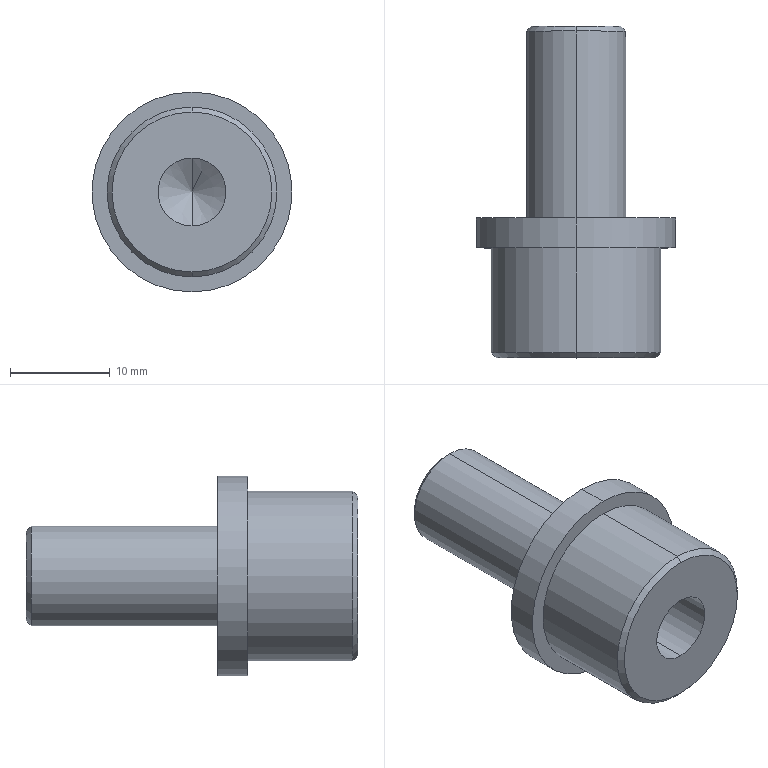Part | SolidWorks | features BaseBody 1 | 1 solid | 18 faces | box 20 x 33.2 x 20 mm | volume 4476 mm3 | cylinder 8 | cone 6 | plane 4 | commonest cylinder face diameters 6.8 x2 10 x2 17 x2 20 x2
STEP:
#1=CARTESIAN_POINT('',(0.,21.7,-5.));
#2=VERTEX_POINT('',#1);
#3=CARTESIAN_POINT('',(0.,21.7,5.));
#4=VERTEX_POINT('',#3);
#5=CARTESIAN_POINT('',(0.,21.7,0.));
#6=DIRECTION('',(0.,-1.,0.));
#7=DIRECTION('',(0.,0.,-1.));
#8=AXIS2_PLACEMENT_3D('',#5,#6,#7);
#9=CIRCLE('',#8,5.);
#10=EDGE_CURVE('',#2,#4,#9,.T.);
#11=ORIENTED_EDGE('',*,*,#10,.T.);
#12=CARTESIAN_POINT('',(0.,3.,5.));
#13=VERTEX_POINT('',#12);
#14=CARTESIAN_POINT('',(0.,22.2,5.));
#15=DIRECTION('',(0.,-1.,0.));
#16=VECTOR('',#15,1000.);
#17=LINE('',#14,#16);
#18=EDGE_CURVE('',#4,#13,#17,.T.);
#19=ORIENTED_EDGE('',*,*,#18,.T.);
#20=CARTESIAN_POINT('',(0.,3.,-5.));
#21=VERTEX_POINT('',#20);
#22=CARTESIAN_POINT('',(0.,3.,0.));
#23=DIRECTION('',(0.,1.,0.));
#24=DIRECTION('',(0.,0.,-1.));
#25=AXIS2_PLACEMENT_3D('',#22,#23,#24);
#26=CIRCLE('',#25,5.);
#27=EDGE_CURVE('',#13,#21,#26,.T.);
#28=ORIENTED_EDGE('',*,*,#27,.T.);
#29=CARTESIAN_POINT('',(0.,22.2,-5.));
#30=DIRECTION('',(0.,-1.,0.));
#31=VECTOR('',#30,1000.);
#32=LINE('',#29,#31);
#33=EDGE_CURVE('',#2,#21,#32,.T.);
#34=ORIENTED_EDGE('',*,*,#33,.F.);
#35=EDGE_LOOP('',(#11,#19,#28,#34));
#36=FACE_OUTER_BOUND('',#35,.T.);
#37=CARTESIAN_POINT('',(0.,22.2,0.));
#38=DIRECTION('',(0.,-1.,0.));
#39=DIRECTION('',(0.,0.,-1.));
#40=AXIS2_PLACEMENT_3D('',#37,#38,#39);
#41=CYLINDRICAL_SURFACE('',#40,5.);
#42=ADVANCED_FACE('',(#36),#41,.T.);
#43=CARTESIAN_POINT('',(0.,22.2,-4.5));
#44=VERTEX_POINT('',#43);
#45=CARTESIAN_POINT('',(0.,22.2,4.5));
#46=VERTEX_POINT('',#45);
#47=CARTESIAN_POINT('',(0.,22.2,0.));
#48=DIRECTION('',(0.,-1.,0.));
#49=DIRECTION('',(0.,0.,-1.));
#50=AXIS2_PLACEMENT_3D('',#47,#48,#49);
#51=CIRCLE('',#50,4.5);
#52=EDGE_CURVE('',#44,#46,#51,.T.);
#53=ORIENTED_EDGE('',*,*,#52,.T.);
#54=CARTESIAN_POINT('',(0.,21.7,5.));
#55=DIRECTION('',(0.,-0.7071,0.7071));
#56=VECTOR('',#55,1000.);
#57=LINE('',#54,#56);
#58=EDGE_CURVE('',#46,#4,#57,.T.);
#59=ORIENTED_EDGE('',*,*,#58,.T.);
#60=ORIENTED_EDGE('',*,*,#10,.F.);
#61=CARTESIAN_POINT('',(0.,21.7,-5.));
#62=DIRECTION('',(0.,-0.7071,-0.7071));
#63=VECTOR('',#62,1000.);
#64=LINE('',#61,#63);
#65=EDGE_CURVE('',#44,#2,#64,.T.);
#66=ORIENTED_EDGE('',*,*,#65,.F.);
#67=EDGE_LOOP('',(#53,#59,#60,#66));
#68=FACE_OUTER_BOUND('',#67,.T.);
#69=CARTESIAN_POINT('',(0.,21.7,0.));
#70=DIRECTION('',(0.,-1.,0.));
#71=DIRECTION('',(0.,0.,-1.));
#72=AXIS2_PLACEMENT_3D('',#69,#70,#71);
#73=CONICAL_SURFACE('',#72,5.,0.7854);
#74=ADVANCED_FACE('',(#68),#73,.T.);
#75=CARTESIAN_POINT('',(0.,3.,10.));
#76=VERTEX_POINT('',#75);
#77=CARTESIAN_POINT('',(0.,3.,-10.));
#78=VERTEX_POINT('',#77);
#79=CARTESIAN_POINT('',(0.,3.,0.));
#80=DIRECTION('',(0.,1.,0.));
#81=DIRECTION('',(0.,0.,-1.));
#82=AXIS2_PLACEMENT_3D('',#79,#80,#81);
#83=CIRCLE('',#82,10.);
#84=EDGE_CURVE('',#76,#78,#83,.T.);
#85=ORIENTED_EDGE('',*,*,#84,.F.);
#86=CARTESIAN_POINT('',(0.,0.,10.));
#87=VERTEX_POINT('',#86);
#88=CARTESIAN_POINT('',(0.,3.,10.));
#89=DIRECTION('',(0.,-1.,0.));
#90=VECTOR('',#89,1000.);
#91=LINE('',#88,#90);
#92=EDGE_CURVE('',#76,#87,#91,.T.);
#93=ORIENTED_EDGE('',*,*,#92,.T.);
#94=CARTESIAN_POINT('',(0.,0.,-10.));
#95=VERTEX_POINT('',#94);
#96=CARTESIAN_POINT('',(0.,0.,0.));
#97=DIRECTION('',(0.,1.,0.));
#98=DIRECTION('',(0.,0.,-1.));
#99=AXIS2_PLACEMENT_3D('',#96,#97,#98);
#100=CIRCLE('',#99,10.);
#101=EDGE_CURVE('',#87,#95,#100,.T.);
#102=ORIENTED_EDGE('',*,*,#101,.T.);
#103=CARTESIAN_POINT('',(0.,3.,-10.));
#104=DIRECTION('',(0.,-1.,0.));
#105=VECTOR('',#104,1000.);
#106=LINE('',#103,#105);
#107=EDGE_CURVE('',#78,#95,#106,.T.);
#108=ORIENTED_EDGE('',*,*,#107,.F.);
#109=EDGE_LOOP('',(#85,#93,#102,#108));
#110=FACE_OUTER_BOUND('',#109,.T.);
#111=CARTESIAN_POINT('',(0.,3.,0.));
#112=DIRECTION('',(0.,-1.,0.));
#113=DIRECTION('',(0.,0.,-1.));
#114=AXIS2_PLACEMENT_3D('',#111,#112,#113);
#115=CYLINDRICAL_SURFACE('',#114,10.);
#116=ADVANCED_FACE('',(#110),#115,.T.);
#117=CARTESIAN_POINT('',(0.,-10.5,8.5));
#118=VERTEX_POINT('',#117);
#119=CARTESIAN_POINT('',(0.,-10.5,-8.5));
#120=VERTEX_POINT('',#119);
#121=CARTESIAN_POINT('',(0.,-10.5,0.));
#122=DIRECTION('',(0.,1.,0.));
#123=DIRECTION('',(0.,0.,1.));
#124=AXIS2_PLACEMENT_3D('',#121,#122,#123);
#125=CIRCLE('',#124,8.5);
#126=EDGE_CURVE('',#118,#120,#125,.T.);
#127=ORIENTED_EDGE('',*,*,#126,.T.);
#128=CARTESIAN_POINT('',(0.,0.,-8.5));
#129=VERTEX_POINT('',#128);
#130=CARTESIAN_POINT('',(0.,-11.,-8.5));
#131=DIRECTION('',(0.,1.,0.));
#132=VECTOR('',#131,1000.);
#133=LINE('',#130,#132);
#134=EDGE_CURVE('',#120,#129,#133,.T.);
#135=ORIENTED_EDGE('',*,*,#134,.T.);
#136=CARTESIAN_POINT('',(0.,0.,8.5));
#137=VERTEX_POINT('',#136);
#138=CARTESIAN_POINT('',(0.,0.,0.));
#139=DIRECTION('',(0.,-1.,0.));
#140=DIRECTION('',(0.,0.,1.));
#141=AXIS2_PLACEMENT_3D('',#138,#139,#140);
#142=CIRCLE('',#141,8.5);
#143=EDGE_CURVE('',#129,#137,#142,.T.);
#144=ORIENTED_EDGE('',*,*,#143,.T.);
#145=CARTESIAN_POINT('',(0.,-11.,8.5));
#146=DIRECTION('',(0.,1.,0.));
#147=VECTOR('',#146,1000.);
#148=LINE('',#145,#147);
#149=EDGE_CURVE('',#118,#137,#148,.T.);
#150=ORIENTED_EDGE('',*,*,#149,.F.);
#151=EDGE_LOOP('',(#127,#135,#144,#150));
#152=FACE_OUTER_BOUND('',#151,.T.);
#153=CARTESIAN_POINT('',(0.,-11.,0.));
#154=DIRECTION('',(0.,1.,0.));
#155=DIRECTION('',(0.,0.,1.));
#156=AXIS2_PLACEMENT_3D('',#153,#154,#155);
#157=CYLINDRICAL_SURFACE('',#156,8.5);
#158=ADVANCED_FACE('',(#152),#157,.T.);
#159=CARTESIAN_POINT('',(0.,-11.,8.));
#160=VERTEX_POINT('',#159);
#161=CARTESIAN_POINT('',(0.,-11.,-8.));
#162=VERTEX_POINT('',#161);
#163=CARTESIAN_POINT('',(0.,-11.,0.));
#164=DIRECTION('',(0.,1.,0.));
#165=DIRECTION('',(0.,0.,1.));
#166=AXIS2_PLACEMENT_3D('',#163,#164,#165);
#167=CIRCLE('',#166,8.);
#168=EDGE_CURVE('',#160,#162,#167,.T.);
#169=ORIENTED_EDGE('',*,*,#168,.T.);
#170=CARTESIAN_POINT('',(0.,-10.5,-8.5));
#171=DIRECTION('',(0.,0.7071,-0.7071));
#172=VECTOR('',#171,1000.);
#173=LINE('',#170,#172);
#174=EDGE_CURVE('',#162,#120,#173,.T.);
#175=ORIENTED_EDGE('',*,*,#174,.T.);
#176=ORIENTED_EDGE('',*,*,#126,.F.);
#177=CARTESIAN_POINT('',(0.,-10.5,8.5));
#178=DIRECTION('',(0.,0.7071,0.7071));
#179=VECTOR('',#178,1000.);
#180=LINE('',#177,#179);
#181=EDGE_CURVE('',#160,#118,#180,.T.);
#182=ORIENTED_EDGE('',*,*,#181,.F.);
#183=EDGE_LOOP('',(#169,#175,#176,#182));
#184=FACE_OUTER_BOUND('',#183,.T.);
#185=CARTESIAN_POINT('',(0.,-10.5,0.));
#186=DIRECTION('',(0.,1.,0.));
#187=DIRECTION('',(0.,0.,1.));
#188=AXIS2_PLACEMENT_3D('',#185,#186,#187);
#189=CONICAL_SURFACE('',#188,8.5,0.7854);
#190=ADVANCED_FACE('',(#184),#189,.T.);
#191=CARTESIAN_POINT('',(0.,1.,3.4));
#192=VERTEX_POINT('',#191);
#193=CARTESIAN_POINT('',(0.,1.,-3.4));
#194=VERTEX_POINT('',#193);
#195=CARTESIAN_POINT('',(0.,1.,0.));
#196=DIRECTION('',(0.,-1.,0.));
#197=DIRECTION('',(0.,0.,-1.));
#198=AXIS2_PLACEMENT_3D('',#195,#196,#197);
#199=CIRCLE('',#198,3.4);
#200=EDGE_CURVE('',#192,#194,#199,.T.);
#201=ORIENTED_EDGE('',*,*,#200,.F.);
#202=CARTESIAN_POINT('',(0.,-11.,3.4));
#203=VERTEX_POINT('',#202);
#204=CARTESIAN_POINT('',(0.,-11.,3.4));
#205=DIRECTION('',(0.,-1.,0.));
#206=VECTOR('',#205,1000.);
#207=LINE('',#204,#206);
#208=EDGE_CURVE('',#192,#203,#207,.T.);
#209=ORIENTED_EDGE('',*,*,#208,.T.);
#210=CARTESIAN_POINT('',(0.,-11.,-3.4));
#211=VERTEX_POINT('',#210);
#212=CARTESIAN_POINT('',(0.,-11.,0.));
#213=DIRECTION('',(0.,1.,0.));
#214=DIRECTION('',(0.,0.,-1.));
#215=AXIS2_PLACEMENT_3D('',#212,#213,#214);
#216=CIRCLE('',#215,3.4);
#217=EDGE_CURVE('',#211,#203,#216,.T.);
#218=ORIENTED_EDGE('',*,*,#217,.F.);
#219=CARTESIAN_POINT('',(0.,-11.,-3.4));
#220=DIRECTION('',(0.,-1.,0.));
#221=VECTOR('',#220,1000.);
#222=LINE('',#219,#221);
#223=EDGE_CURVE('',#194,#211,#222,.T.);
#224=ORIENTED_EDGE('',*,*,#223,.F.);
#225=EDGE_LOOP('',(#201,#209,#218,#224));
#226=FACE_OUTER_BOUND('',#225,.T.);
#227=CARTESIAN_POINT('',(0.,-11.,0.));
#228=DIRECTION('',(0.,-1.,0.));
#229=DIRECTION('',(0.,0.,-1.));
#230=AXIS2_PLACEMENT_3D('',#227,#228,#229);
#231=CYLINDRICAL_SURFACE('',#230,3.4);
#232=ADVANCED_FACE('',(#226),#231,.F.);
#233=CARTESIAN_POINT('',(0.,3.043,0.));
#234=VERTEX_POINT('',#233);
#235=CARTESIAN_POINT('',(0.,1.,-3.4));
#236=DIRECTION('',(0.,-0.515,-0.8572));
#237=VECTOR('',#236,1000.);
#238=LINE('',#235,#237);
#239=EDGE_CURVE('',#234,#194,#238,.T.);
#240=ORIENTED_EDGE('',*,*,#239,.F.);
#241=CARTESIAN_POINT('',(0.,1.,3.4));
#242=DIRECTION('',(0.,-0.515,0.8572));
#243=VECTOR('',#242,1000.);
#244=LINE('',#241,#243);
#245=EDGE_CURVE('',#234,#192,#244,.T.);
#246=ORIENTED_EDGE('',*,*,#245,.T.);
#247=ORIENTED_EDGE('',*,*,#200,.T.);
#248=EDGE_LOOP('',(#240,#246,#247));
#249=FACE_OUTER_BOUND('',#248,.T.);
#250=CARTESIAN_POINT('',(0.,1.,0.));
#251=DIRECTION('',(0.,-1.,0.));
#252=DIRECTION('',(0.,0.,-1.));
#253=AXIS2_PLACEMENT_3D('',#250,#251,#252);
#254=CONICAL_SURFACE('',#253,3.4,1.03);
#255=ADVANCED_FACE('',(#249),#254,.F.);
#256=ORIENTED_EDGE('',*,*,#18,.F.);
#257=CARTESIAN_POINT('',(0.,21.7,0.));
#258=DIRECTION('',(0.,-1.,0.));
#259=DIRECTION('',(0.,0.,-1.));
#260=AXIS2_PLACEMENT_3D('',#257,#258,#259);
#261=CIRCLE('',#260,5.);
#262=EDGE_CURVE('',#4,#2,#261,.T.);
#263=ORIENTED_EDGE('',*,*,#262,.T.);
#264=ORIENTED_EDGE('',*,*,#33,.T.);
#265=CARTESIAN_POINT('',(0.,3.,0.));
#266=DIRECTION('',(0.,1.,0.));
#267=DIRECTION('',(0.,0.,-1.));
#268=AXIS2_PLACEMENT_3D('',#265,#266,#267);
#269=CIRCLE('',#268,5.);
#270=EDGE_CURVE('',#21,#13,#269,.T.);
#271=ORIENTED_EDGE('',*,*,#270,.T.);
#272=EDGE_LOOP('',(#256,#263,#264,#271));
#273=FACE_OUTER_BOUND('',#272,.T.);
#274=CARTESIAN_POINT('',(0.,22.2,0.));
#275=DIRECTION('',(0.,-1.,0.));
#276=DIRECTION('',(0.,0.,-1.));
#277=AXIS2_PLACEMENT_3D('',#274,#275,#276);
#278=CYLINDRICAL_SURFACE('',#277,5.);
#279=ADVANCED_FACE('',(#273),#278,.T.);
#280=CARTESIAN_POINT('',(0.,3.,0.));
#281=DIRECTION('',(0.,1.,0.));
#282=DIRECTION('',(0.,0.,-1.));
#283=AXIS2_PLACEMENT_3D('',#280,#281,#282);
#284=CIRCLE('',#283,10.);
#285=EDGE_CURVE('',#78,#76,#284,.T.);
#286=ORIENTED_EDGE('',*,*,#285,.T.);
#287=ORIENTED_EDGE('',*,*,#84,.T.);
#288=EDGE_LOOP('',(#286,#287));
#289=FACE_OUTER_BOUND('',#288,.T.);
#290=ORIENTED_EDGE('',*,*,#270,.F.);
#291=ORIENTED_EDGE('',*,*,#27,.F.);
#292=EDGE_LOOP('',(#290,#291));
#293=FACE_BOUND('',#292,.T.);
#294=CARTESIAN_POINT('',(0.,3.,0.));
#295=DIRECTION('',(0.,1.,0.));
#296=DIRECTION('',(0.,0.,1.));
#297=AXIS2_PLACEMENT_3D('',#294,#295,#296);
#298=PLANE('',#297);
#299=ADVANCED_FACE('',(#289,#293),#298,.T.);
#300=ORIENTED_EDGE('',*,*,#58,.F.);
#301=CARTESIAN_POINT('',(0.,22.2,0.));
#302=DIRECTION('',(0.,-1.,0.));
#303=DIRECTION('',(0.,0.,-1.));
#304=AXIS2_PLACEMENT_3D('',#301,#302,#303);
#305=CIRCLE('',#304,4.5);
#306=EDGE_CURVE('',#46,#44,#305,.T.);
#307=ORIENTED_EDGE('',*,*,#306,.T.);
#308=ORIENTED_EDGE('',*,*,#65,.T.);
#309=ORIENTED_EDGE('',*,*,#262,.F.);
#310=EDGE_LOOP('',(#300,#307,#308,#309));
#311=FACE_OUTER_BOUND('',#310,.T.);
#312=CARTESIAN_POINT('',(0.,21.7,0.));
#313=DIRECTION('',(0.,-1.,0.));
#314=DIRECTION('',(0.,0.,-1.));
#315=AXIS2_PLACEMENT_3D('',#312,#313,#314);
#316=CONICAL_SURFACE('',#315,5.,0.7854);
#317=ADVANCED_FACE('',(#311),#316,.T.);
#318=ORIENTED_EDGE('',*,*,#92,.F.);
#319=ORIENTED_EDGE('',*,*,#285,.F.);
#320=ORIENTED_EDGE('',*,*,#107,.T.);
#321=CARTESIAN_POINT('',(0.,0.,0.));
#322=DIRECTION('',(0.,1.,0.));
#323=DIRECTION('',(0.,0.,-1.));
#324=AXIS2_PLACEMENT_3D('',#321,#322,#323);
#325=CIRCLE('',#324,10.);
#326=EDGE_CURVE('',#95,#87,#325,.T.);
#327=ORIENTED_EDGE('',*,*,#326,.T.);
#328=EDGE_LOOP('',(#318,#319,#320,#327));
#329=FACE_OUTER_BOUND('',#328,.T.);
#330=CARTESIAN_POINT('',(0.,3.,0.));
#331=DIRECTION('',(0.,-1.,0.));
#332=DIRECTION('',(0.,0.,-1.));
#333=AXIS2_PLACEMENT_3D('',#330,#331,#332);
#334=CYLINDRICAL_SURFACE('',#333,10.);
#335=ADVANCED_FACE('',(#329),#334,.T.);
#336=ORIENTED_EDGE('',*,*,#52,.F.);
#337=ORIENTED_EDGE('',*,*,#306,.F.);
#338=EDGE_LOOP('',(#336,#337));
#339=FACE_OUTER_BOUND('',#338,.T.);
#340=CARTESIAN_POINT('',(0.,22.2,0.));
#341=DIRECTION('',(0.,1.,0.));
#342=DIRECTION('',(0.,0.,1.));
#343=AXIS2_PLACEMENT_3D('',#340,#341,#342);
#344=PLANE('',#343);
#345=ADVANCED_FACE('',(#339),#344,.T.);
#346=ORIENTED_EDGE('',*,*,#326,.F.);
#347=ORIENTED_EDGE('',*,*,#101,.F.);
#348=EDGE_LOOP('',(#346,#347));
#349=FACE_OUTER_BOUND('',#348,.T.);
#350=CARTESIAN_POINT('',(0.,0.,0.));
#351=DIRECTION('',(0.,-1.,0.));
#352=DIRECTION('',(0.,0.,1.));
#353=AXIS2_PLACEMENT_3D('',#350,#351,#352);
#354=CIRCLE('',#353,8.5);
#355=EDGE_CURVE('',#137,#129,#354,.T.);
#356=ORIENTED_EDGE('',*,*,#355,.F.);
#357=ORIENTED_EDGE('',*,*,#143,.F.);
#358=EDGE_LOOP('',(#356,#357));
#359=FACE_BOUND('',#358,.T.);
#360=CARTESIAN_POINT('',(0.,0.,0.));
#361=DIRECTION('',(0.,1.,0.));
#362=DIRECTION('',(0.,0.,1.));
#363=AXIS2_PLACEMENT_3D('',#360,#361,#362);
#364=PLANE('',#363);
#365=ADVANCED_FACE('',(#349,#359),#364,.F.);
#366=ORIENTED_EDGE('',*,*,#134,.F.);
#367=CARTESIAN_POINT('',(0.,-10.5,0.));
#368=DIRECTION('',(0.,1.,0.));
#369=DIRECTION('',(0.,0.,1.));
#370=AXIS2_PLACEMENT_3D('',#367,#368,#369);
#371=CIRCLE('',#370,8.5);
#372=EDGE_CURVE('',#120,#118,#371,.T.);
#373=ORIENTED_EDGE('',*,*,#372,.T.);
#374=ORIENTED_EDGE('',*,*,#149,.T.);
#375=ORIENTED_EDGE('',*,*,#355,.T.);
#376=EDGE_LOOP('',(#366,#373,#374,#375));
#377=FACE_OUTER_BOUND('',#376,.T.);
#378=CARTESIAN_POINT('',(0.,-11.,0.));
#379=DIRECTION('',(0.,1.,0.));
#380=DIRECTION('',(0.,0.,1.));
#381=AXIS2_PLACEMENT_3D('',#378,#379,#380);
#382=CYLINDRICAL_SURFACE('',#381,8.5);
#383=ADVANCED_FACE('',(#377),#382,.T.);
#384=ORIENTED_EDGE('',*,*,#174,.F.);
#385=CARTESIAN_POINT('',(0.,-11.,0.));
#386=DIRECTION('',(0.,1.,0.));
#387=DIRECTION('',(0.,0.,1.));
#388=AXIS2_PLACEMENT_3D('',#385,#386,#387);
#389=CIRCLE('',#388,8.);
#390=EDGE_CURVE('',#162,#160,#389,.T.);
#391=ORIENTED_EDGE('',*,*,#390,.T.);
#392=ORIENTED_EDGE('',*,*,#181,.T.);
#393=ORIENTED_EDGE('',*,*,#372,.F.);
#394=EDGE_LOOP('',(#384,#391,#392,#393));
#395=FACE_OUTER_BOUND('',#394,.T.);
#396=CARTESIAN_POINT('',(0.,-10.5,0.));
#397=DIRECTION('',(0.,1.,0.));
#398=DIRECTION('',(0.,0.,1.));
#399=AXIS2_PLACEMENT_3D('',#396,#397,#398);
#400=CONICAL_SURFACE('',#399,8.5,0.7854);
#401=ADVANCED_FACE('',(#395),#400,.T.);
#402=ORIENTED_EDGE('',*,*,#217,.T.);
#403=CARTESIAN_POINT('',(0.,-11.,0.));
#404=DIRECTION('',(0.,1.,0.));
#405=DIRECTION('',(0.,0.,-1.));
#406=AXIS2_PLACEMENT_3D('',#403,#404,#405);
#407=CIRCLE('',#406,3.4);
#408=EDGE_CURVE('',#203,#211,#407,.T.);
#409=ORIENTED_EDGE('',*,*,#408,.T.);
#410=EDGE_LOOP('',(#402,#409));
#411=FACE_BOUND('',#410,.T.);
#412=ORIENTED_EDGE('',*,*,#168,.F.);
#413=ORIENTED_EDGE('',*,*,#390,.F.);
#414=EDGE_LOOP('',(#412,#413));
#415=FACE_OUTER_BOUND('',#414,.T.);
#416=CARTESIAN_POINT('',(0.,-11.,0.));
#417=DIRECTION('',(0.,-1.,0.));
#418=DIRECTION('',(0.,0.,-1.));
#419=AXIS2_PLACEMENT_3D('',#416,#417,#418);
#420=PLANE('',#419);
#421=ADVANCED_FACE('',(#411,#415),#420,.T.);
#422=ORIENTED_EDGE('',*,*,#208,.F.);
#423=CARTESIAN_POINT('',(0.,1.,0.));
#424=DIRECTION('',(0.,-1.,0.));
#425=DIRECTION('',(0.,0.,-1.));
#426=AXIS2_PLACEMENT_3D('',#423,#424,#425);
#427=CIRCLE('',#426,3.4);
#428=EDGE_CURVE('',#194,#192,#427,.T.);
#429=ORIENTED_EDGE('',*,*,#428,.F.);
#430=ORIENTED_EDGE('',*,*,#223,.T.);
#431=ORIENTED_EDGE('',*,*,#408,.F.);
#432=EDGE_LOOP('',(#422,#429,#430,#431));
#433=FACE_OUTER_BOUND('',#432,.T.);
#434=CARTESIAN_POINT('',(0.,-11.,0.));
#435=DIRECTION('',(0.,-1.,0.));
#436=DIRECTION('',(0.,0.,-1.));
#437=AXIS2_PLACEMENT_3D('',#434,#435,#436);
#438=CYLINDRICAL_SURFACE('',#437,3.4);
#439=ADVANCED_FACE('',(#433),#438,.F.);
#440=ORIENTED_EDGE('',*,*,#245,.F.);
#441=ORIENTED_EDGE('',*,*,#239,.T.);
#442=ORIENTED_EDGE('',*,*,#428,.T.);
#443=EDGE_LOOP('',(#440,#441,#442));
#444=FACE_OUTER_BOUND('',#443,.T.);
#445=CARTESIAN_POINT('',(0.,1.,0.));
#446=DIRECTION('',(0.,-1.,0.));
#447=DIRECTION('',(0.,0.,-1.));
#448=AXIS2_PLACEMENT_3D('',#445,#446,#447);
#449=CONICAL_SURFACE('',#448,3.4,1.03);
#450=ADVANCED_FACE('',(#444),#449,.F.);
#451=CLOSED_SHELL('',(#42,#74,#116,#158,#190,#232,#255,#279,#299,#317,#335,#345,#365,#383,#401,#421,#439,#450));
#452=MANIFOLD_SOLID_BREP('',#451);
#453=CARTESIAN_POINT('',(0.,0.,0.));
#454=DIRECTION('',(0.,0.,1.));
#455=DIRECTION('',(1.,0.,0.));
#456=AXIS2_PLACEMENT_3D('',#453,#454,#455);
#457=(LENGTH_UNIT()NAMED_UNIT(*)SI_UNIT(.MILLI.,.METRE.));
#458=UNCERTAINTY_MEASURE_WITH_UNIT(LENGTH_MEASURE(0.00001),#457,'','');
#459=(NAMED_UNIT(*)PLANE_ANGLE_UNIT()SI_UNIT($,.RADIAN.));
#460=(NAMED_UNIT(*)SI_UNIT($,.STERADIAN.)SOLID_ANGLE_UNIT());
#461=(GEOMETRIC_REPRESENTATION_CONTEXT(3)GLOBAL_UNCERTAINTY_ASSIGNED_CONTEXT((#458))GLOBAL_UNIT_ASSIGNED_CONTEXT((#457,#459,#460))REPRESENTATION_CONTEXT('',''));
#462=ADVANCED_BREP_SHAPE_REPRESENTATION('',(#452,#456),#461);